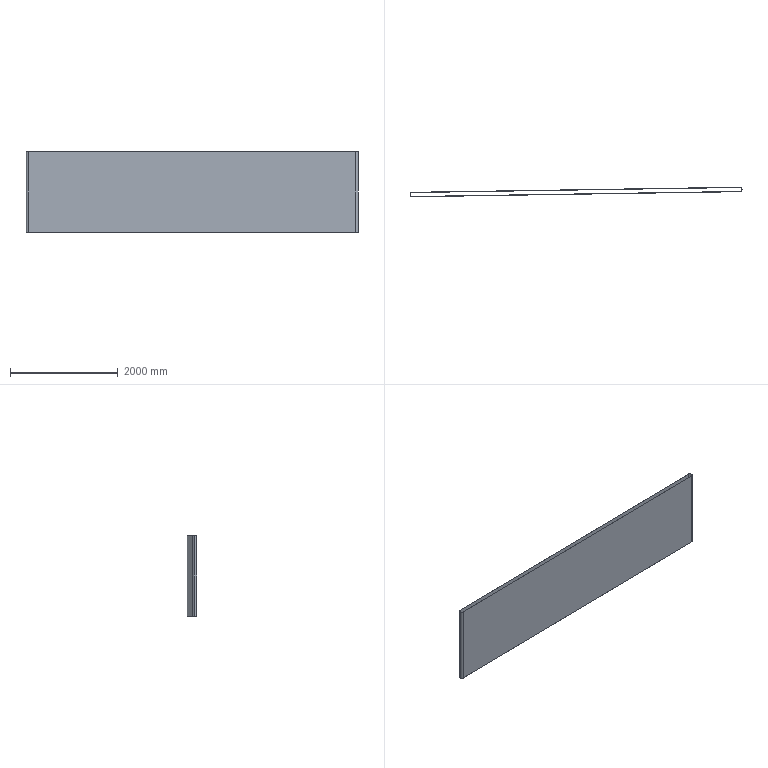Part | STEP file | Microwave Drying Flat Conveyor-dai | 1 solid | 18 faces | box 6157 x 175.545 x 1500 mm | volume 52078468 mm3 | plane 12 | cylinder 6 | commonest cylinder face diameters 75.388 x3 80.988 x3
STEP:
#1=CARTESIAN_POINT('',(-3075.826,-47.278,750.));
#2=VERTEX_POINT('',#1);
#3=CARTESIAN_POINT('',(-3038.719,-9.589,750.));
#4=VERTEX_POINT('',#3);
#5=CARTESIAN_POINT('',(-3038.132,-47.278,750.));
#6=DIRECTION('',(0.,0.,-1.));
#7=DIRECTION('',(0.01556,-0.9999,0.));
#8=AXIS2_PLACEMENT_3D('',#5,#6,#7);
#9=CIRCLE('',#8,37.694);
#10=EDGE_CURVE('',#2,#4,#9,.T.);
#11=ORIENTED_EDGE('',*,*,#10,.F.);
#12=CARTESIAN_POINT('',(-3075.826,-47.278,-750.));
#13=VERTEX_POINT('',#12);
#14=CARTESIAN_POINT('',(-3075.826,-47.278,0.));
#15=DIRECTION('',(0.,0.,-1.));
#16=VECTOR('',#15,1000.);
#17=LINE('',#14,#16);
#18=EDGE_CURVE('',#2,#13,#17,.T.);
#19=ORIENTED_EDGE('',*,*,#18,.T.);
#20=CARTESIAN_POINT('',(-3038.719,-9.589,-750.));
#21=VERTEX_POINT('',#20);
#22=CARTESIAN_POINT('',(-3038.132,-47.278,-750.));
#23=DIRECTION('',(0.,0.,-1.));
#24=DIRECTION('',(0.01556,-0.9999,0.));
#25=AXIS2_PLACEMENT_3D('',#22,#23,#24);
#26=CIRCLE('',#25,37.694);
#27=EDGE_CURVE('',#13,#21,#26,.T.);
#28=ORIENTED_EDGE('',*,*,#27,.T.);
#29=CARTESIAN_POINT('',(-3038.719,-9.589,750.));
#30=DIRECTION('',(0.,0.,-1.));
#31=VECTOR('',#30,1000.);
#32=LINE('',#29,#31);
#33=EDGE_CURVE('',#4,#21,#32,.T.);
#34=ORIENTED_EDGE('',*,*,#33,.F.);
#35=EDGE_LOOP('',(#11,#19,#28,#34));
#36=FACE_OUTER_BOUND('',#35,.T.);
#37=CARTESIAN_POINT('',(-3038.132,-47.278,0.));
#38=DIRECTION('',(0.,0.,-1.));
#39=DIRECTION('',(-1.,0.,0.));
#40=AXIS2_PLACEMENT_3D('',#37,#38,#39);
#41=CYLINDRICAL_SURFACE('',#40,37.694);
#42=ADVANCED_FACE('',(#36),#41,.F.);
#43=CARTESIAN_POINT('',(-3037.502,-87.767,750.));
#44=VERTEX_POINT('',#43);
#45=CARTESIAN_POINT('',(-3078.626,-47.278,750.));
#46=VERTEX_POINT('',#45);
#47=CARTESIAN_POINT('',(-3038.132,-47.278,750.));
#48=DIRECTION('',(0.,0.,-1.));
#49=DIRECTION('',(0.01556,-0.9999,0.));
#50=AXIS2_PLACEMENT_3D('',#47,#48,#49);
#51=CIRCLE('',#50,40.494);
#52=EDGE_CURVE('',#44,#46,#51,.T.);
#53=ORIENTED_EDGE('',*,*,#52,.T.);
#54=CARTESIAN_POINT('',(-3078.626,-47.278,-750.));
#55=VERTEX_POINT('',#54);
#56=CARTESIAN_POINT('',(-3078.626,-47.278,0.));
#57=DIRECTION('',(0.,0.,-1.));
#58=VECTOR('',#57,1000.);
#59=LINE('',#56,#58);
#60=EDGE_CURVE('',#46,#55,#59,.T.);
#61=ORIENTED_EDGE('',*,*,#60,.T.);
#62=CARTESIAN_POINT('',(-3037.502,-87.767,-750.));
#63=VERTEX_POINT('',#62);
#64=CARTESIAN_POINT('',(-3038.132,-47.278,-750.));
#65=DIRECTION('',(0.,0.,-1.));
#66=DIRECTION('',(0.01556,-0.9999,0.));
#67=AXIS2_PLACEMENT_3D('',#64,#65,#66);
#68=CIRCLE('',#67,40.494);
#69=EDGE_CURVE('',#63,#55,#68,.T.);
#70=ORIENTED_EDGE('',*,*,#69,.F.);
#71=CARTESIAN_POINT('',(-3037.502,-87.767,750.));
#72=DIRECTION('',(0.,0.,1.));
#73=VECTOR('',#72,1000.);
#74=LINE('',#71,#73);
#75=EDGE_CURVE('',#63,#44,#74,.T.);
#76=ORIENTED_EDGE('',*,*,#75,.T.);
#77=EDGE_LOOP('',(#53,#61,#70,#76));
#78=FACE_OUTER_BOUND('',#77,.T.);
#79=CARTESIAN_POINT('',(-3038.132,-47.278,0.));
#80=DIRECTION('',(0.,0.,-1.));
#81=DIRECTION('',(-1.,0.,0.));
#82=AXIS2_PLACEMENT_3D('',#79,#80,#81);
#83=CYLINDRICAL_SURFACE('',#82,40.494);
#84=ADVANCED_FACE('',(#78),#83,.T.);
#85=CARTESIAN_POINT('',(-3038.762,-6.789,-750.));
#86=VERTEX_POINT('',#85);
#87=CARTESIAN_POINT('',(3037.502,87.767,-750.));
#88=VERTEX_POINT('',#87);
#89=CARTESIAN_POINT('',(-3038.762,-6.789,-750.));
#90=DIRECTION('',(0.9999,0.01556,0.));
#91=VECTOR('',#90,1000.);
#92=LINE('',#89,#91);
#93=EDGE_CURVE('',#86,#88,#92,.T.);
#94=ORIENTED_EDGE('',*,*,#93,.F.);
#95=CARTESIAN_POINT('',(-3038.762,-6.789,750.));
#96=VERTEX_POINT('',#95);
#97=CARTESIAN_POINT('',(-3038.762,-6.789,750.));
#98=DIRECTION('',(0.,0.,1.));
#99=VECTOR('',#98,1000.);
#100=LINE('',#97,#99);
#101=EDGE_CURVE('',#86,#96,#100,.T.);
#102=ORIENTED_EDGE('',*,*,#101,.T.);
#103=CARTESIAN_POINT('',(3037.502,87.767,750.));
#104=VERTEX_POINT('',#103);
#105=CARTESIAN_POINT('',(-3038.762,-6.789,750.));
#106=DIRECTION('',(0.9999,0.01556,0.));
#107=VECTOR('',#106,1000.);
#108=LINE('',#105,#107);
#109=EDGE_CURVE('',#96,#104,#108,.T.);
#110=ORIENTED_EDGE('',*,*,#109,.T.);
#111=CARTESIAN_POINT('',(3037.502,87.767,750.));
#112=DIRECTION('',(0.,0.,1.));
#113=VECTOR('',#112,1000.);
#114=LINE('',#111,#113);
#115=EDGE_CURVE('',#88,#104,#114,.T.);
#116=ORIENTED_EDGE('',*,*,#115,.F.);
#117=EDGE_LOOP('',(#94,#102,#110,#116));
#118=FACE_OUTER_BOUND('',#117,.T.);
#119=CARTESIAN_POINT('',(-3038.762,-6.789,750.));
#120=DIRECTION('',(-0.01556,0.9999,0.));
#121=DIRECTION('',(-0.9999,-0.01556,0.));
#122=AXIS2_PLACEMENT_3D('',#119,#120,#121);
#123=PLANE('',#122);
#124=ADVANCED_FACE('',(#118),#123,.T.);
#125=CARTESIAN_POINT('',(3037.546,84.968,-750.));
#126=VERTEX_POINT('',#125);
#127=CARTESIAN_POINT('',(-3038.719,-9.589,-750.));
#128=DIRECTION('',(0.9999,0.01556,0.));
#129=VECTOR('',#128,1000.);
#130=LINE('',#127,#129);
#131=EDGE_CURVE('',#21,#126,#130,.T.);
#132=ORIENTED_EDGE('',*,*,#131,.F.);
#133=CARTESIAN_POINT('',(-3038.762,-6.789,-750.));
#134=DIRECTION('',(-0.01556,0.9999,0.));
#135=VECTOR('',#134,1000.);
#136=LINE('',#133,#135);
#137=EDGE_CURVE('',#21,#86,#136,.T.);
#138=ORIENTED_EDGE('',*,*,#137,.T.);
#139=ORIENTED_EDGE('',*,*,#93,.T.);
#140=CARTESIAN_POINT('',(3037.502,87.767,-750.));
#141=DIRECTION('',(-0.01556,0.9999,0.));
#142=VECTOR('',#141,1000.);
#143=LINE('',#140,#142);
#144=EDGE_CURVE('',#126,#88,#143,.T.);
#145=ORIENTED_EDGE('',*,*,#144,.F.);
#146=EDGE_LOOP('',(#132,#138,#139,#145));
#147=FACE_OUTER_BOUND('',#146,.T.);
#148=CARTESIAN_POINT('',(-3038.762,-6.789,-750.));
#149=DIRECTION('',(0.,0.,-1.));
#150=DIRECTION('',(-1.,0.,0.));
#151=AXIS2_PLACEMENT_3D('',#148,#149,#150);
#152=PLANE('',#151);
#153=ADVANCED_FACE('',(#147),#152,.T.);
#154=CARTESIAN_POINT('',(3037.546,84.968,750.));
#155=VERTEX_POINT('',#154);
#156=CARTESIAN_POINT('',(-3038.719,-9.589,750.));
#157=DIRECTION('',(0.9999,0.01556,0.));
#158=VECTOR('',#157,1000.);
#159=LINE('',#156,#158);
#160=EDGE_CURVE('',#4,#155,#159,.T.);
#161=ORIENTED_EDGE('',*,*,#160,.F.);
#162=ORIENTED_EDGE('',*,*,#33,.T.);
#163=ORIENTED_EDGE('',*,*,#131,.T.);
#164=CARTESIAN_POINT('',(3037.546,84.968,750.));
#165=DIRECTION('',(0.,0.,-1.));
#166=VECTOR('',#165,1000.);
#167=LINE('',#164,#166);
#168=EDGE_CURVE('',#155,#126,#167,.T.);
#169=ORIENTED_EDGE('',*,*,#168,.F.);
#170=EDGE_LOOP('',(#161,#162,#163,#169));
#171=FACE_OUTER_BOUND('',#170,.T.);
#172=CARTESIAN_POINT('',(-3038.719,-9.589,750.));
#173=DIRECTION('',(0.01556,-0.9999,0.));
#174=DIRECTION('',(0.9999,0.01556,0.));
#175=AXIS2_PLACEMENT_3D('',#172,#173,#174);
#176=PLANE('',#175);
#177=ADVANCED_FACE('',(#171),#176,.T.);
#178=ORIENTED_EDGE('',*,*,#60,.F.);
#179=CARTESIAN_POINT('',(-3038.132,-47.278,750.));
#180=DIRECTION('',(0.,0.,-1.));
#181=DIRECTION('',(0.01556,-0.9999,0.));
#182=AXIS2_PLACEMENT_3D('',#179,#180,#181);
#183=CIRCLE('',#182,40.494);
#184=EDGE_CURVE('',#46,#96,#183,.T.);
#185=ORIENTED_EDGE('',*,*,#184,.T.);
#186=ORIENTED_EDGE('',*,*,#101,.F.);
#187=CARTESIAN_POINT('',(-3038.132,-47.278,-750.));
#188=DIRECTION('',(0.,0.,-1.));
#189=DIRECTION('',(0.01556,-0.9999,0.));
#190=AXIS2_PLACEMENT_3D('',#187,#188,#189);
#191=CIRCLE('',#190,40.494);
#192=EDGE_CURVE('',#55,#86,#191,.T.);
#193=ORIENTED_EDGE('',*,*,#192,.F.);
#194=EDGE_LOOP('',(#178,#185,#186,#193));
#195=FACE_OUTER_BOUND('',#194,.T.);
#196=CARTESIAN_POINT('',(-3038.132,-47.278,0.));
#197=DIRECTION('',(0.,0.,-1.));
#198=DIRECTION('',(-1.,0.,0.));
#199=AXIS2_PLACEMENT_3D('',#196,#197,#198);
#200=CYLINDRICAL_SURFACE('',#199,40.494);
#201=ADVANCED_FACE('',(#195),#200,.T.);
#202=ORIENTED_EDGE('',*,*,#69,.T.);
#203=ORIENTED_EDGE('',*,*,#192,.T.);
#204=ORIENTED_EDGE('',*,*,#137,.F.);
#205=ORIENTED_EDGE('',*,*,#27,.F.);
#206=CARTESIAN_POINT('',(-3037.546,-84.968,-750.));
#207=VERTEX_POINT('',#206);
#208=CARTESIAN_POINT('',(-3038.132,-47.278,-750.));
#209=DIRECTION('',(0.,0.,-1.));
#210=DIRECTION('',(0.01556,-0.9999,0.));
#211=AXIS2_PLACEMENT_3D('',#208,#209,#210);
#212=CIRCLE('',#211,37.694);
#213=EDGE_CURVE('',#207,#13,#212,.T.);
#214=ORIENTED_EDGE('',*,*,#213,.F.);
#215=CARTESIAN_POINT('',(-3037.502,-87.767,-750.));
#216=DIRECTION('',(0.01556,-0.9999,0.));
#217=VECTOR('',#216,1000.);
#218=LINE('',#215,#217);
#219=EDGE_CURVE('',#207,#63,#218,.T.);
#220=ORIENTED_EDGE('',*,*,#219,.T.);
#221=EDGE_LOOP('',(#202,#203,#204,#205,#214,#220));
#222=FACE_OUTER_BOUND('',#221,.T.);
#223=CARTESIAN_POINT('',(-3037.502,-87.767,-750.));
#224=DIRECTION('',(0.,0.,-1.));
#225=DIRECTION('',(-1.,0.,0.));
#226=AXIS2_PLACEMENT_3D('',#223,#224,#225);
#227=PLANE('',#226);
#228=ADVANCED_FACE('',(#222),#227,.T.);
#229=ORIENTED_EDGE('',*,*,#18,.F.);
#230=CARTESIAN_POINT('',(-3037.546,-84.968,750.));
#231=VERTEX_POINT('',#230);
#232=CARTESIAN_POINT('',(-3038.132,-47.278,750.));
#233=DIRECTION('',(0.,0.,-1.));
#234=DIRECTION('',(0.01556,-0.9999,0.));
#235=AXIS2_PLACEMENT_3D('',#232,#233,#234);
#236=CIRCLE('',#235,37.694);
#237=EDGE_CURVE('',#231,#2,#236,.T.);
#238=ORIENTED_EDGE('',*,*,#237,.F.);
#239=CARTESIAN_POINT('',(-3037.546,-84.968,750.));
#240=DIRECTION('',(0.,0.,-1.));
#241=VECTOR('',#240,1000.);
#242=LINE('',#239,#241);
#243=EDGE_CURVE('',#231,#207,#242,.T.);
#244=ORIENTED_EDGE('',*,*,#243,.T.);
#245=ORIENTED_EDGE('',*,*,#213,.T.);
#246=EDGE_LOOP('',(#229,#238,#244,#245));
#247=FACE_OUTER_BOUND('',#246,.T.);
#248=CARTESIAN_POINT('',(-3038.132,-47.278,0.));
#249=DIRECTION('',(0.,0.,-1.));
#250=DIRECTION('',(-1.,0.,0.));
#251=AXIS2_PLACEMENT_3D('',#248,#249,#250);
#252=CYLINDRICAL_SURFACE('',#251,37.694);
#253=ADVANCED_FACE('',(#247),#252,.F.);
#254=ORIENTED_EDGE('',*,*,#237,.T.);
#255=ORIENTED_EDGE('',*,*,#10,.T.);
#256=CARTESIAN_POINT('',(-3038.762,-6.789,750.));
#257=DIRECTION('',(0.01556,-0.9999,0.));
#258=VECTOR('',#257,1000.);
#259=LINE('',#256,#258);
#260=EDGE_CURVE('',#96,#4,#259,.T.);
#261=ORIENTED_EDGE('',*,*,#260,.F.);
#262=ORIENTED_EDGE('',*,*,#184,.F.);
#263=ORIENTED_EDGE('',*,*,#52,.F.);
#264=CARTESIAN_POINT('',(-3037.502,-87.767,750.));
#265=DIRECTION('',(-0.01556,0.9999,0.));
#266=VECTOR('',#265,1000.);
#267=LINE('',#264,#266);
#268=EDGE_CURVE('',#44,#231,#267,.T.);
#269=ORIENTED_EDGE('',*,*,#268,.T.);
#270=EDGE_LOOP('',(#254,#255,#261,#262,#263,#269));
#271=FACE_OUTER_BOUND('',#270,.T.);
#272=CARTESIAN_POINT('',(-3037.502,-87.767,750.));
#273=DIRECTION('',(0.,0.,1.));
#274=DIRECTION('',(1.,0.,0.));
#275=AXIS2_PLACEMENT_3D('',#272,#273,#274);
#276=PLANE('',#275);
#277=ADVANCED_FACE('',(#271),#276,.T.);
#278=ORIENTED_EDGE('',*,*,#75,.F.);
#279=CARTESIAN_POINT('',(3038.762,6.789,-750.));
#280=VERTEX_POINT('',#279);
#281=CARTESIAN_POINT('',(3038.762,6.789,-750.));
#282=DIRECTION('',(-0.9999,-0.01556,0.));
#283=VECTOR('',#282,1000.);
#284=LINE('',#281,#283);
#285=EDGE_CURVE('',#280,#63,#284,.T.);
#286=ORIENTED_EDGE('',*,*,#285,.F.);
#287=CARTESIAN_POINT('',(3038.762,6.789,750.));
#288=VERTEX_POINT('',#287);
#289=CARTESIAN_POINT('',(3038.762,6.789,750.));
#290=DIRECTION('',(0.,0.,1.));
#291=VECTOR('',#290,1000.);
#292=LINE('',#289,#291);
#293=EDGE_CURVE('',#280,#288,#292,.T.);
#294=ORIENTED_EDGE('',*,*,#293,.T.);
#295=CARTESIAN_POINT('',(3038.762,6.789,750.));
#296=DIRECTION('',(-0.9999,-0.01556,0.));
#297=VECTOR('',#296,1000.);
#298=LINE('',#295,#297);
#299=EDGE_CURVE('',#288,#44,#298,.T.);
#300=ORIENTED_EDGE('',*,*,#299,.T.);
#301=EDGE_LOOP('',(#278,#286,#294,#300));
#302=FACE_OUTER_BOUND('',#301,.T.);
#303=CARTESIAN_POINT('',(3038.762,6.789,750.));
#304=DIRECTION('',(0.01556,-0.9999,0.));
#305=DIRECTION('',(0.9999,0.01556,0.));
#306=AXIS2_PLACEMENT_3D('',#303,#304,#305);
#307=PLANE('',#306);
#308=ADVANCED_FACE('',(#302),#307,.T.);
#309=ORIENTED_EDGE('',*,*,#285,.T.);
#310=ORIENTED_EDGE('',*,*,#219,.F.);
#311=CARTESIAN_POINT('',(3038.719,9.589,-750.));
#312=VERTEX_POINT('',#311);
#313=CARTESIAN_POINT('',(3038.719,9.589,-750.));
#314=DIRECTION('',(-0.9999,-0.01556,0.));
#315=VECTOR('',#314,1000.);
#316=LINE('',#313,#315);
#317=EDGE_CURVE('',#312,#207,#316,.T.);
#318=ORIENTED_EDGE('',*,*,#317,.F.);
#319=CARTESIAN_POINT('',(3038.762,6.789,-750.));
#320=DIRECTION('',(0.01556,-0.9999,0.));
#321=VECTOR('',#320,1000.);
#322=LINE('',#319,#321);
#323=EDGE_CURVE('',#312,#280,#322,.T.);
#324=ORIENTED_EDGE('',*,*,#323,.T.);
#325=EDGE_LOOP('',(#309,#310,#318,#324));
#326=FACE_OUTER_BOUND('',#325,.T.);
#327=CARTESIAN_POINT('',(3038.762,6.789,-750.));
#328=DIRECTION('',(0.,0.,-1.));
#329=DIRECTION('',(-1.,0.,0.));
#330=AXIS2_PLACEMENT_3D('',#327,#328,#329);
#331=PLANE('',#330);
#332=ADVANCED_FACE('',(#326),#331,.T.);
#333=ORIENTED_EDGE('',*,*,#317,.T.);
#334=ORIENTED_EDGE('',*,*,#243,.F.);
#335=CARTESIAN_POINT('',(3038.719,9.589,750.));
#336=VERTEX_POINT('',#335);
#337=CARTESIAN_POINT('',(3038.719,9.589,750.));
#338=DIRECTION('',(-0.9999,-0.01556,0.));
#339=VECTOR('',#338,1000.);
#340=LINE('',#337,#339);
#341=EDGE_CURVE('',#336,#231,#340,.T.);
#342=ORIENTED_EDGE('',*,*,#341,.F.);
#343=CARTESIAN_POINT('',(3038.719,9.589,750.));
#344=DIRECTION('',(0.,0.,-1.));
#345=VECTOR('',#344,1000.);
#346=LINE('',#343,#345);
#347=EDGE_CURVE('',#336,#312,#346,.T.);
#348=ORIENTED_EDGE('',*,*,#347,.T.);
#349=EDGE_LOOP('',(#333,#334,#342,#348));
#350=FACE_OUTER_BOUND('',#349,.T.);
#351=CARTESIAN_POINT('',(3038.719,9.589,750.));
#352=DIRECTION('',(-0.01556,0.9999,0.));
#353=DIRECTION('',(-0.9999,-0.01556,0.));
#354=AXIS2_PLACEMENT_3D('',#351,#352,#353);
#355=PLANE('',#354);
#356=ADVANCED_FACE('',(#350),#355,.T.);
#357=ORIENTED_EDGE('',*,*,#341,.T.);
#358=ORIENTED_EDGE('',*,*,#268,.F.);
#359=ORIENTED_EDGE('',*,*,#299,.F.);
#360=CARTESIAN_POINT('',(3038.762,6.789,750.));
#361=DIRECTION('',(-0.01556,0.9999,0.));
#362=VECTOR('',#361,1000.);
#363=LINE('',#360,#362);
#364=EDGE_CURVE('',#288,#336,#363,.T.);
#365=ORIENTED_EDGE('',*,*,#364,.T.);
#366=EDGE_LOOP('',(#357,#358,#359,#365));
#367=FACE_OUTER_BOUND('',#366,.T.);
#368=CARTESIAN_POINT('',(3038.762,6.789,750.));
#369=DIRECTION('',(0.,0.,1.));
#370=DIRECTION('',(1.,0.,0.));
#371=AXIS2_PLACEMENT_3D('',#368,#369,#370);
#372=PLANE('',#371);
#373=ADVANCED_FACE('',(#367),#372,.T.);
#374=ORIENTED_EDGE('',*,*,#293,.F.);
#375=CARTESIAN_POINT('',(3038.132,47.278,-750.));
#376=DIRECTION('',(0.,0.,-1.));
#377=DIRECTION('',(-0.01556,0.9999,0.));
#378=AXIS2_PLACEMENT_3D('',#375,#376,#377);
#379=CIRCLE('',#378,40.494);
#380=EDGE_CURVE('',#88,#280,#379,.T.);
#381=ORIENTED_EDGE('',*,*,#380,.F.);
#382=ORIENTED_EDGE('',*,*,#115,.T.);
#383=CARTESIAN_POINT('',(3038.132,47.278,750.));
#384=DIRECTION('',(0.,0.,-1.));
#385=DIRECTION('',(-0.01556,0.9999,0.));
#386=AXIS2_PLACEMENT_3D('',#383,#384,#385);
#387=CIRCLE('',#386,40.494);
#388=EDGE_CURVE('',#104,#288,#387,.T.);
#389=ORIENTED_EDGE('',*,*,#388,.T.);
#390=EDGE_LOOP('',(#374,#381,#382,#389));
#391=FACE_OUTER_BOUND('',#390,.T.);
#392=CARTESIAN_POINT('',(3038.132,47.278,0.));
#393=DIRECTION('',(0.,0.,-1.));
#394=DIRECTION('',(-1.,0.,0.));
#395=AXIS2_PLACEMENT_3D('',#392,#393,#394);
#396=CYLINDRICAL_SURFACE('',#395,40.494);
#397=ADVANCED_FACE('',(#391),#396,.T.);
#398=ORIENTED_EDGE('',*,*,#380,.T.);
#399=ORIENTED_EDGE('',*,*,#323,.F.);
#400=CARTESIAN_POINT('',(3038.132,47.278,-750.));
#401=DIRECTION('',(0.,0.,-1.));
#402=DIRECTION('',(-0.01556,0.9999,0.));
#403=AXIS2_PLACEMENT_3D('',#400,#401,#402);
#404=CIRCLE('',#403,37.694);
#405=EDGE_CURVE('',#126,#312,#404,.T.);
#406=ORIENTED_EDGE('',*,*,#405,.F.);
#407=ORIENTED_EDGE('',*,*,#144,.T.);
#408=EDGE_LOOP('',(#398,#399,#406,#407));
#409=FACE_OUTER_BOUND('',#408,.T.);
#410=CARTESIAN_POINT('',(3037.502,87.767,-750.));
#411=DIRECTION('',(0.,0.,-1.));
#412=DIRECTION('',(-1.,0.,0.));
#413=AXIS2_PLACEMENT_3D('',#410,#411,#412);
#414=PLANE('',#413);
#415=ADVANCED_FACE('',(#409),#414,.T.);
#416=ORIENTED_EDGE('',*,*,#405,.T.);
#417=ORIENTED_EDGE('',*,*,#347,.F.);
#418=CARTESIAN_POINT('',(3038.132,47.278,750.));
#419=DIRECTION('',(0.,0.,-1.));
#420=DIRECTION('',(-0.01556,0.9999,0.));
#421=AXIS2_PLACEMENT_3D('',#418,#419,#420);
#422=CIRCLE('',#421,37.694);
#423=EDGE_CURVE('',#155,#336,#422,.T.);
#424=ORIENTED_EDGE('',*,*,#423,.F.);
#425=ORIENTED_EDGE('',*,*,#168,.T.);
#426=EDGE_LOOP('',(#416,#417,#424,#425));
#427=FACE_OUTER_BOUND('',#426,.T.);
#428=CARTESIAN_POINT('',(3038.132,47.278,0.));
#429=DIRECTION('',(0.,0.,-1.));
#430=DIRECTION('',(-1.,0.,0.));
#431=AXIS2_PLACEMENT_3D('',#428,#429,#430);
#432=CYLINDRICAL_SURFACE('',#431,37.694);
#433=ADVANCED_FACE('',(#427),#432,.F.);
#434=ORIENTED_EDGE('',*,*,#423,.T.);
#435=ORIENTED_EDGE('',*,*,#364,.F.);
#436=ORIENTED_EDGE('',*,*,#388,.F.);
#437=CARTESIAN_POINT('',(3037.502,87.767,750.));
#438=DIRECTION('',(0.01556,-0.9999,0.));
#439=VECTOR('',#438,1000.);
#440=LINE('',#437,#439);
#441=EDGE_CURVE('',#104,#155,#440,.T.);
#442=ORIENTED_EDGE('',*,*,#441,.T.);
#443=EDGE_LOOP('',(#434,#435,#436,#442));
#444=FACE_OUTER_BOUND('',#443,.T.);
#445=CARTESIAN_POINT('',(3037.502,87.767,750.));
#446=DIRECTION('',(0.,0.,1.));
#447=DIRECTION('',(1.,0.,0.));
#448=AXIS2_PLACEMENT_3D('',#445,#446,#447);
#449=PLANE('',#448);
#450=ADVANCED_FACE('',(#444),#449,.T.);
#451=ORIENTED_EDGE('',*,*,#260,.T.);
#452=ORIENTED_EDGE('',*,*,#160,.T.);
#453=ORIENTED_EDGE('',*,*,#441,.F.);
#454=ORIENTED_EDGE('',*,*,#109,.F.);
#455=EDGE_LOOP('',(#451,#452,#453,#454));
#456=FACE_OUTER_BOUND('',#455,.T.);
#457=CARTESIAN_POINT('',(-3038.762,-6.789,750.));
#458=DIRECTION('',(0.,0.,1.));
#459=DIRECTION('',(1.,0.,0.));
#460=AXIS2_PLACEMENT_3D('',#457,#458,#459);
#461=PLANE('',#460);
#462=ADVANCED_FACE('',(#456),#461,.T.);
#463=CLOSED_SHELL('',(#42,#84,#124,#153,#177,#201,#228,#253,#277,#308,#332,#356,#373,#397,#415,#433,#450,#462));
#464=MANIFOLD_SOLID_BREP('',#463);
#465=CARTESIAN_POINT('',(0.,0.,0.));
#466=DIRECTION('',(0.,0.,1.));
#467=DIRECTION('',(1.,0.,0.));
#468=AXIS2_PLACEMENT_3D('',#465,#466,#467);
#469=(LENGTH_UNIT()NAMED_UNIT(*)SI_UNIT(.MILLI.,.METRE.));
#470=UNCERTAINTY_MEASURE_WITH_UNIT(LENGTH_MEASURE(0.00001),#469,'','');
#471=(NAMED_UNIT(*)PLANE_ANGLE_UNIT()SI_UNIT($,.RADIAN.));
#472=(NAMED_UNIT(*)SI_UNIT($,.STERADIAN.)SOLID_ANGLE_UNIT());
#473=(GEOMETRIC_REPRESENTATION_CONTEXT(3)GLOBAL_UNCERTAINTY_ASSIGNED_CONTEXT((#470))GLOBAL_UNIT_ASSIGNED_CONTEXT((#469,#471,#472))REPRESENTATION_CONTEXT('',''));
#474=ADVANCED_BREP_SHAPE_REPRESENTATION('',(#464,#468),#473);